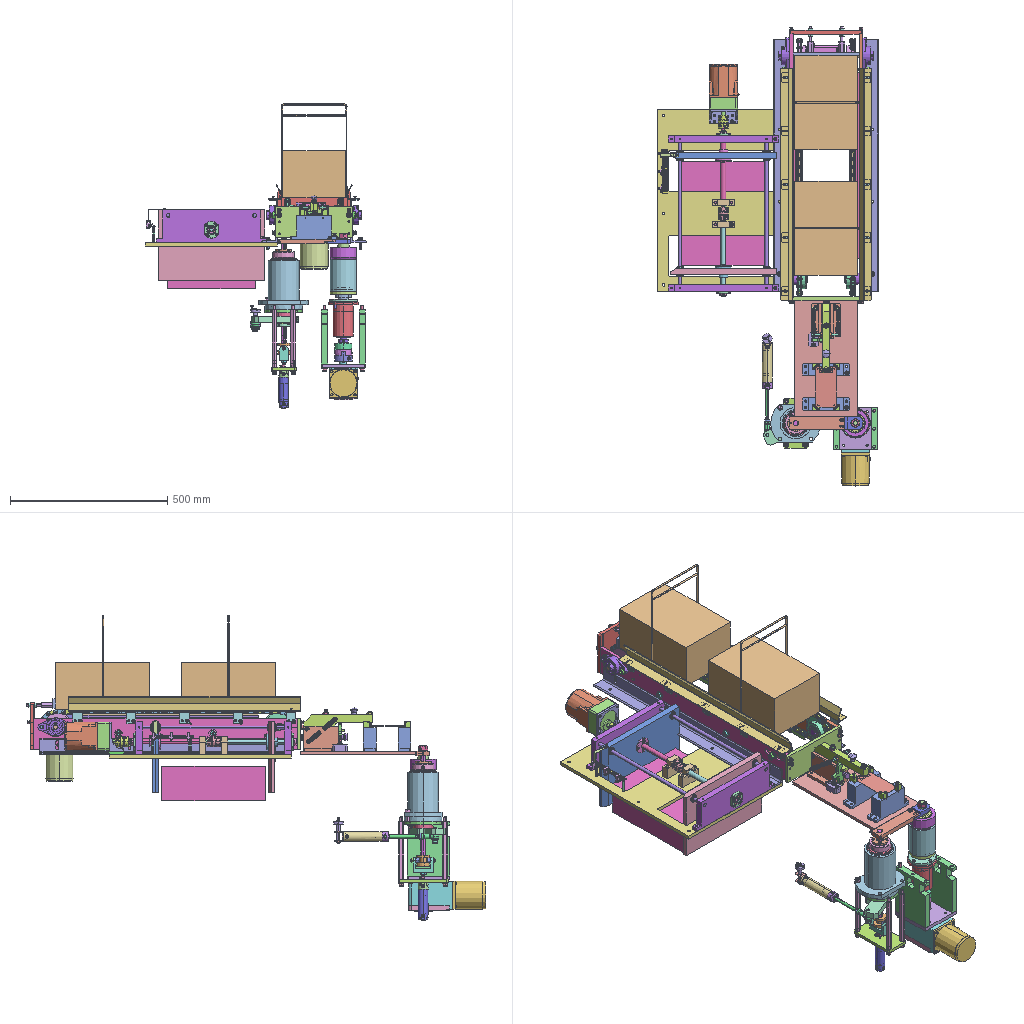Assembly | STEP file | 219 different items | 577 placed | box 704 x 1463 x 971 mm
Parts list (item | name | quantity | parent item | size | volume):
1 | 0217_205_Base_Plate | x1 | - | 200 x 370 x 10 mm | 736866 mm3
2 | 0217_207_Base | x2 | - | 150 x 40 x 75 mm | 343539 mm3
3 | 0217_017_WGDLJ-20-5-5 | x4 | - | 20 x 20 x 20 mm | 5354 mm3
4 | 0217_012_WSRPM20_40_20 | x1 | - | 40 x 20 x 5 mm | 3328 mm3
5 | 0217_002_WR18-20 | x2 | - | 19 x 4.5 x 19 mm | 92.511 mm3
6 | 0217_Z_AWA12-100 | x4 | in 0217_001_AWA12-100 | 13.1 x 13.1 x 53.1 mm | 757.901 mm3
7 | 0217_206_Base | x1 | in _0217_SA01 | 30 x 45 x 20 mm | 23102 mm3
8 | 0217_204_Block | x1 | in _0217_SA01 | 45 x 9.9 x 82 mm | 15419 mm3
9 | 0217_Z_PJL8-10-1 | x1 | in 0217_013_PJL8-10 | 43 x 8 x 8 mm | 1284 mm3
10 | 0217_Z_PJL8-10-2 | x1 | in 0217_013_PJL8-10 | 20 x 4.8 x 4.8 mm | 157.602 mm3
11 | 0217_003_DBTS6-10-10 | x1 | in _0217_SA01 | 24 x 16 x 16 mm | 1816 mm3
12 | 0217_301_SCB6-20 | x4 | in _0217_SA01, _0217_SA02 | 26 x 10 x 10 mm | 952.027 mm3
13 | 0217_306_SNTRCS8 | x1 | in _0217_SA01 | 4 x 15.011 x 13 mm | 435.9 mm3
14 | 0217_201_Base | x1 | in _0217_SA02 | 90 x 110 x 80 mm | 389355 mm3
15 | 0217_004_MPBZ15-10 | x2 | in _0217_SA02 | 10 x 21 x 21 mm | 1565 mm3
16 | 0217_Z_SBSP8-30-1 | x2 | in 0217_015_SBSPO8-30 | 30 x 8 x 8 mm | 1385 mm3
17 | 0217_Z_SBSP8-30-2 | x2 | in 0217_015_SBSPO8-30 | 6.8 x 15.011 x 13 mm | 746.792 mm3
18 | 0217_302_SLW6 | x3 | in _0217_SA02 | 1.5 x 12.2 x 12.2 mm | 128.756 mm3
19 | 0217_303_PFW6 | x3 | in _0217_SA02 | 1.6 x 12.5 x 12.5 mm | 141.61 mm3
20 | 0217_203_Shaft | x1 | in _0217_SA03 | 20 x 147 x 20 mm | 23227 mm3
21 | 0217_005_WSSS25-15-1 | x1 | in _0217_SA03 | 1 x 25 x 25 mm | 282.743 mm3
22 | 0217_006_WSSS25-8-1 | x1 | in _0217_SA03 | 1 x 25 x 25 mm | 414.69 mm3
23 | 0217_007_NOOS8-16 | x1 | in _0217_SA03 | 22 x 30 x 30 mm | 5015 mm3
24 | 0217_202_Arm | x1 | in _0217_SA04 | 20 x 220 x 54 mm | 161429 mm3
25 | 0217_016_MPFZU8-10 | x2 | in _0217_SA04 | 10 x 14 x 14 mm | 412.979 mm3
26 | 0217_Z_SBSPO8-45-1 | x2 | in 0217_014_SBSPO8-45 | 45 x 8 x 8 mm | 2139 mm3
27 | 0217_Z_SBSPO8-45-2 | x2 | in 0217_014_SBSPO8-45 | 6.8 x 15.011 x 13 mm | 746.792 mm3
28 | 0217_011_NMM6-25 | x1 | in _0217_SA04 | 25 x 32 x 25 mm | 5504 mm3
29 | 0217_Z_ANBNS10-80-1 | x1 | in 0217_010_ANBNS10_80 | 80 x 10 x 10 mm | 6095 mm3
30 | 0217_Z_ANBNS10-80-2 | x1 | in 0217_010_ANBNS10_80 | 6 x 19.6 x 17 mm | 1146 mm3
31 | 0217_Z_PUSS10-40-1 | x1 | in 0217_009_PUSS10-40 | 46 x 10 x 10 mm | 3323 mm3
32 | 0217_Z_PUSS10-40-2 | x1 | in 0217_009_PUSS10-40 | 6 x 19.63 x 17 mm | 1142 mm3
33 | 0217_Z_SCCG8-55-1 | x1 | in 0217_008_SCCG8-55 | 61 x 8 x 8 mm | 3039 mm3
34 | 0217_Z_SCCG8-55-2 | x2 | in 0217_008_SCCG8-55 | 0.8 x 14 x 11.95 mm | 51.564 mm3
35 | 0217_Work-A | x1 | - | 65 x 130 x 0.7 mm | 5915 mm3
36 | 0217_304_SCB3-25 | x4 | - | 28 x 5.5 x 5.5 mm | 238.258 mm3
37 | 0217_305_SFBJ6-12 | x1 | - | 12 x 12 x 12 mm | 419.433 mm3
38 | 0228_001_SRBN25-A | x4 | in _0228_SA01-1, _0228_SA01-2 | 25 x 1.6 x 25 mm | 333.381 mm3
39 | 0228_002_MSB12-25 | x4 | in _0228_SA01-1, _0228_SA01-2 | 45 x 17 x 17 mm | 5025 mm3
40 | 0228_Z_LGTS40-590-K4-P1601 | x2 | in 0228_006_LGTS40-590-K4-P160 | 17 x 14 x 590 mm | 119990 mm3
41 | 0228_Z_LGTS40-590-K4-P1602 | x2 | in 0228_006_LGTS40-590-K4-P160 | 20 x 10 x 590 mm | 38370 mm3
42 | 0228_007_STWN25 | x2 | in _0228_SA01-1, _0228_SA01-2 | 1.2 x 31.3 x 28.55 mm | 254.107 mm3
43 | 0228_009_SB6905ZZ | x4 | in _0228_SA01-1, _0228_SA01-2 | 9 x 42 x 42 mm | 7312 mm3
44 | 0228_Z_Chain_RF2040SSS-441 | x68 | in 0228_103_Chain_RF2040SSS-44 | 18.2 x 12 x 37.4 mm | 1630 mm3
45 | 0228_Z_Chain_RF2040SSS-442 | x68 | in 0228_103_Chain_RF2040SSS-44 | 10.95 x 12 x 37.4 mm | 1766 mm3
46 | 0228_104_Sprocket_RF2040S1200 | x2 | in _0228_SA01-1, _0228_SA01-2 | 103.209 x 103.209 x 25 mm | 105106 mm3
47 | 0228_105_Sprocket_RF2040S1200 | x2 | in _0228_SA01-1, _0228_SA01-2 | 103.209 x 103.209 x 25 mm | 79551 mm3
48 | 0228_201_Plate | x1 | in _0228_SA01-1 | 12 x 100 x 840 mm | 978760 mm3
49 | 0228_203_Bracket | x2 | in _0228_SA01-1, _0228_SA01-2 | 50 x 50 x 800 mm | 373941 mm3
50 | 0228_206_Guide | x2 | in _0228_SA01-1, _0228_SA01-2 | 6 x 18 x 600 mm | 64069 mm3
51 | 0228_207_Bracket | x2 | in _0228_SA01-1, _0228_SA01-2 | 30 x 30 x 590 mm | 100045 mm3
52 | 0228_210_Bracket | x10 | in _0228_SA01-1, _0228_SA01-2 | 25 x 40 x 30 mm | 5273 mm3
53 | 0228_211_Guide | x2 | in _0228_SA01-1, _0228_SA01-2 | 38 x 46.651 x 740 mm | 124477 mm3
54 | 0228_214_Shaft | x2 | in _0228_SA01-1, _0228_SA01-2 | 77.35 x 35 x 35 mm | 35572 mm3
55 | 0228_215_Post | x8 | in _0228_SA01-1, _0228_SA01-2 | 26 x 13.856 x 12 mm | 2134 mm3
56 | 0228_301_ACB8-100 | x2 | in _0228_SA01-1, _0228_SA01-2 | 108 x 13 x 13 mm | 5949 mm3
57 | socket head cap screw_iso_ISO 4762 M8 x 30 --- 30N | x2 | in _0228_SA01-1, _0228_SA01-2 | 38 x 13 x 13 mm | 2418 mm3
58 | socket head cap screw_iso_ISO 4762 M8 x 20 --- 20N | x2 | in _0228_SA01-1, _0228_SA01-2 | 28 x 13 x 13 mm | 1915 mm3
59 | 0228_305_MSSFS5-8 | x4 | in _0228_SA01-1, _0228_SA01-2 | 8 x 5 x 5 mm | 139.331 mm3
60 | 0228_308_SCB5-15 | x14 | in _0228_SA01-1, _0228_SA01-2 | 20 x 8.5 x 8.5 mm | 536.391 mm3
61 | socket head cap screw_iso_ISO 4762 M5 x 12 --- 12N | x2 | in _0228_SA01-1, _0228_SA01-2 | 17 x 8.5 x 8.5 mm | 476.406 mm3
62 | socket head cap screw_iso_ISO 4762 M4 x 8 --- 8N | x2 | in _0228_SA01-1, _0228_SA01-2 | 12 x 7 x 7 mm | 234.975 mm3
63 | 0228_311_LBNR12 | x2 | in _0228_SA01-1, _0228_SA01-2 | 10 x 21.9 x 19 mm | 2286 mm3
64 | 0228_313_SPWF12 | x2 | in _0228_SA01-1, _0228_SA01-2 | 2.5 x 24 x 24 mm | 799.143 mm3
65 | 0228_314_SPWF8 | x6 | in _0228_SA01-1, _0228_SA01-2 | 1.6 x 17 x 17 mm | 274.5 mm3
66 | 0228_316_SPWF5 | x14 | in _0228_SA01-1, _0228_SA01-2 | 1 x 10 x 10 mm | 56.478 mm3
67 | 0228_317_SPWF4 | x2 | in _0228_SA01-1, _0228_SA01-2 | 0.8 x 9 x 9 mm | 39.276 mm3
68 | 0228_318_SSLW12 | x2 | in _0228_SA01-1, _0228_SA01-2 | 3 x 21.5 x 21.494 mm | 721.153 mm3
69 | 0228_319_SSLW8 | x4 | in _0228_SA01-1, _0228_SA01-2 | 2 x 15.4 x 15.396 mm | 260.908 mm3
70 | 0228_321_SSLW5 | x16 | in _0228_SA01-1, _0228_SA01-2 | 1.3 x 9.2 x 9.198 mm | 58.481 mm3
71 | 0228_322_SSLW4 | x2 | in _0228_SA01-1, _0228_SA01-2 | 1 x 7.6 x 7.598 mm | 31.433 mm3
72 | 0228_202_Plate | x1 | in _0228_SA01-2 | 12 x 100 x 840 mm | 978079 mm3
73 | 0228_003_MSB12-10 | x1 | in _0228_SA02 | 30 x 17 x 17 mm | 3328 mm3
74 | 0228_004_SLSBG19-48-M10-N8 | x1 | in _0228_SA02 | 63 x 21.939 x 19 mm | 15277 mm3
75 | 0228_Z_HDH151 | x2 | in 0228_008_HDH15 | 113 x 60 x 33.3 mm | 71474 mm3
76 | 0228_Z_HDH152 | x2 | in 0228_008_HDH15 | 7.128 x 7.128 x 6 mm | 118.77 mm3
77 | 0228_Z_HDH153 | x2 | in 0228_008_HDH15 | 6 x 5 x 6 mm | 118.77 mm3
78 | 0228_010_KES5-25 | x3 | in _0228_SA02 | 25 x 5 x 5 mm | 594.343 mm3
79 | 0228_101_Motor_5RK40GN-C | x1 | in _0228_SA02 | 137 x 90 x 90 mm | 667092 mm3
80 | 0228_Z_Gearhead_5GN120RH1 | x1 | in 0228_102_Gearhead_5GN120RH | 107 x 104 x 93 mm | 637231 mm3
81 | 0228_Z_Gearhead_5GN120RH2 | x1 | in 0228_102_Gearhead_5GN120RH | 25 x 25 x 83 mm | 25062 mm3
82 | 0228_205_Shaft | x1 | in _0228_SA02 | 305 x 15 x 15 mm | 52825 mm3
83 | 0228_213_Arm | x1 | in _0228_SA02 | 9 x 78 x 135 mm | 88772 mm3
84 | socket head cap screw_iso_ISO 4762 M10 x 25 --- 25N | x2 | in _0228_SA02 | 35 x 16 x 16 mm | 3616 mm3
85 | socket head cap screw_iso_ISO 4762 M6 x 20 --- 20N | x5 | in _0228_SA02, _0228_Assy | 26 x 10 x 10 mm | 956.582 mm3
86 | 0228_315_SPWF6 | x5 | in _0228_SA02, _0228_Assy | 1.6 x 12.5 x 12.5 mm | 144.878 mm3
87 | 0228_320_SSLW6 | x5 | in _0228_SA02, _0228_Assy | 1.5 x 12.2 x 12.197 mm | 128.674 mm3
88 | 0228_005_SLSBH17-35-F50-M8-N6 | x2 | in _0228_Assy | 85 x 19.63 x 17 mm | 10911 mm3
89 | 0228_204_Shaft | x2 | in _0228_Assy | 210 x 20 x 20 mm | 61901 mm3
90 | 0228_208_Plate | x1 | in _0228_Assy | 234 x 150 x 12 mm | 410826 mm3
91 | 0228_209_Stopper | x1 | in _0228_Assy | 210 x 30 x 9 mm | 55294 mm3
92 | 0228_212_Plate | x1 | in _0228_Assy | 243 x 100 x 12 mm | 281737 mm3
93 | 0228_307_SCB6-15 | x2 | in _0228_Assy | 21 x 10 x 10 mm | 817.284 mm3
94 | 0228_312_SHNJ-M8 | x4 | in _0228_Assy | 6.5 x 15.011 x 13 mm | 713.151 mm3
95 | 0228_Work-A | x2 | in _0228_Assy | 209.998 x 299.999 x 300 mm | 9019523 mm3
96 | 0229_Z_SCSBS20-24_1 | x1 | in 0229_004_SCSBS20-24 | 32 x 32 x 15 mm | 5310 mm3
97 | 0229_Z_SCSBS20-24_2 | x1 | in 0229_004_SCSBS20-24 | 6 x 5 x 6 mm | 115.41 mm3
98 | 0229_Z_SCSBS20-24_3 | x1 | in 0229_004_SCSBS20-24 | 5 x 6 x 6 mm | 115.41 mm3
99 | 0229_Z_B6204ZZNR_1 | x2 | in 0229_007_B6204ZZNR | 14 x 47 x 47 mm | 18805 mm3
100 | 0229_Z_B6204ZZNR_2 | x2 | in 0229_007_B6204ZZNR | 1.12 x 52.6 x 52.7 mm | 674.018 mm3
101 | 0229_Z_MFJC55-20-22_1 | x1 | in 0229_010_MFJC55-20-22 | 17 x 55 x 55 mm | 22049 mm3
102 | 0229_Z_MFJC55-20-22_2 | x1 | in 0229_010_MFJC55-20-22 | 30 x 55 x 54.982 mm | 40722 mm3
103 | 0229_Z_MFJC55-20-22_3 | x1 | in 0229_010_MFJC55-20-22 | 10 x 30.82 x 10 mm | 1082 mm3
104 | 0229_Z_MFJC55-20-22_4 | x1 | in 0229_010_MFJC55-20-22 | 30 x 54.982 x 55 mm | 39507 mm3
105 | 0229_Z_MFJC55-20-22_5 | x1 | in 0229_010_MFJC55-20-22 | 10 x 10 x 30.82 mm | 1082 mm3
106 | 0229_Z_5IK40AW-GAL20J_1 | x1 | in 0229_101_Servo_Motor_5IK40AW-GAL20J | 150 x 90 x 140 mm | 1226880 mm3
107 | 0229_Z_5IK40AW-GAL20J_2 | x1 | in 0229_101_Servo_Motor_5IK40AW-GAL20J | 90 x 93.5 x 105 mm | 664924 mm3
108 | 0229_201_Plate | x1 | in _0229_SA01 | 135 x 12 x 140 mm | 188675 mm3
109 | 0229_202_Plate | x2 | in _0229_SA01 | 135 x 173 x 20 mm | 406809 mm3
110 | 0229_211_Holder | x1 | in _0229_SA01 | 95 x 110 x 95 mm | 199422 mm3
111 | 0229_213_Shaft | x1 | in _0229_SA01 | 50 x 184 x 50 mm | 77662 mm3
112 | 0229_214_Holder | x1 | in _0229_SA01 | 85 x 10 x 85 mm | 51385 mm3
113 | 0229_215_Holder | x1 | in _0229_SA01 | 78 x 22 x 78 mm | 64740 mm3
114 | 0229_220_Holder | x1 | in _0229_SA01 | 89 x 8 x 89 mm | 33937 mm3
115 | 0229_302_M5x12 | x1 | in _0229_SA01 | 17 x 8.5 x 8.5 mm | 476.423 mm3
116 | 0229_306_M6x16 | x1 | in _0229_SA01 | 22 x 10 x 10 mm | 843.509 mm3
117 | 0229_307_M6x20 | x2 | in _0229_SA01 | 26 x 10 x 10 mm | 956.605 mm3
118 | 0229_309_M8x30 | x4 | in _0229_SA01 | 38 x 13 x 13 mm | 2418 mm3
119 | 0229_315_SPWF8 | x8 | in _0229_SA01, _0229_SA02 | 1.6 x 17 x 17 mm | 274.5 mm3
120 | 0229_317_SSLW6 | x2 | in _0229_SA01, _0229_SA02 | 1.5 x 12.2 x 12.197 mm | 128.674 mm3
121 | 0229_318_SSLW8 | x8 | in _0229_SA01, _0229_SA02 | 2 x 15.4 x 15.396 mm | 260.908 mm3
122 | 0229_Z_PHSC10A_1 | x1 | in 0229_001_PHSC10A | - | 7061 mm3
123 | 0229_Z_PHSC10A_2 | x1 | in 0229_001_PHSC10A | - | 2169 mm3
124 | 0229_Z_CFUA6-16_1 | x2 | in 0229_002_CFUA6-16 | 28 x 15.999 x 16 mm | 2735 mm3
125 | 0229_Z_CFUA6-16_2 | x2 | in 0229_002_CFUA6-16 | 5.2 x 11.547 x 10 mm | 345.697 mm3
126 | 0229_Z_SCCN50-22_1 | x1 | in 0229_003_SCCN50-22 | 22 x 70 x 70 mm | 36768 mm3
127 | 0229_Z_SCCN50-22_2 | x1 | in 0229_003_SCCN50-22 | 10 x 8 x 10 mm | 459 mm3
128 | 0229_Z_SCCN50-22_3 | x1 | in 0229_003_SCCN50-22 | 10 x 10 x 8 mm | 459.001 mm3
129 | 0229_005_STWN30 | x1 | in _0229_SA02 | 1.5 x 36.9 x 33.85 mm | 424.063 mm3
130 | 0229_006_STWN10 | x1 | in _0229_SA02 | 1 x 14.4 x 12.3 mm | 59.275 mm3
131 | 0229_Z_B6010ZZNR_1 | x2 | in 0229_008_B6010ZZNR | 16 x 80 x 80 mm | 45982 mm3
132 | 0229_Z_B6010ZZNR_2 | x2 | in 0229_008_B6010ZZNR | 1.7 x 86.435 x 86.6 mm | 2077 mm3
133 | 0229_009_B6206ZZ | x2 | in _0229_SA02 | 16 x 62 x 62 mm | 35690 mm3
134 | 0229_Z_BSFM16-335-M8-NTW_1 | x1 | in 0229_011_BSFM16-335-M8-NTW | 16.6 x 16.559 x 335 mm | 69757 mm3
135 | 0229_Z_BSFM16-335-M8-NTW_2 | x1 | in 0229_011_BSFM16-335-M8-NTW | 51 x 51 x 50 mm | 33822 mm3
136 | 0229_Z_BSFM16-335-M8-NTW_3 | x1 | in 0229_011_BSFM16-335-M8-NTW | 51 x 51 x 50 mm | 33822 mm3
137 | 0229_Z_Cylinder_CG1BN25-50_1 | x1 | in 0229_102_Cylinder_CG1BN25-50 | 31 x 100 x 31 mm | 43980 mm3
138 | 0229_Z_Cylinder_CG1BN25-50_2 | x1 | in 0229_102_Cylinder_CG1BN25-50 | 31.4 x 23 x 31.4 mm | 12893 mm3
139 | 0229_Z_Cylinder_CG1BN25-50_3 | x1 | in 0229_102_Cylinder_CG1BN25-50 | 24.9 x 137.5 x 24.9 mm | 12725 mm3
140 | 0229_Z_Cylinder_CG1BN25-50_4 | x1 | in 0229_102_Cylinder_CG1BN25-50 | 19.6 x 6 x 17 mm | 1151 mm3
141 | 0229_Z_Cylinder_CG1DN25-75_1 | x1 | in 0229_103_Cylinder_CG1DN25-75 | 31 x 31 x 125 mm | 50538 mm3
142 | 0229_Z_Cylinder_CG1DN25-75_2 | x1 | in 0229_103_Cylinder_CG1DN25-75 | 31.4 x 31.4 x 23 mm | 12832 mm3
143 | 0229_Z_Cylinder_CG1DN25-75_3 | x1 | in 0229_103_Cylinder_CG1DN25-75 | 24.9 x 24.9 x 162.5 mm | 14688 mm3
144 | 0229_Z_Cylinder_CG1DN25-75_4 | x1 | in 0229_103_Cylinder_CG1DN25-75 | 33 x 31 x 29 mm | 5061 mm3
145 | 0229_Z_Cylinder_CG1DN25-75_5 | x1 | in 0229_103_Cylinder_CG1DN25-75 | 19.6 x 6 x 17 mm | 1151 mm3
146 | 0229_203_Plate | x1 | in _0229_SA02 | 160 x 10 x 80 mm | 122466 mm3
147 | 0229_204_Stud | x4 | in _0229_SA02 | 16.166 x 198.5 x 14 mm | 31042 mm3
148 | 0229_205_Joint | x1 | in _0229_SA02 | 64 x 48 x 30 mm | 41736 mm3
149 | 0229_206_Joint | x1 | in _0229_SA02 | 40 x 35 x 40 mm | 25414 mm3
150 | 0229_207_Pin | x1 | in _0229_SA02 | 30 x 73 x 30 mm | 11176 mm3
151 | 0229_208_Holder | x1 | in _0229_SA02 | 120 x 10 x 120 mm | 60495 mm3
152 | 0229_209_Color | x1 | in _0229_SA02 | 56 x 15.2 x 56 mm | 7593 mm3
153 | 0229_210_Holder | x1 | in _0229_SA02 | 120 x 157 x 160 mm | 628932 mm3
154 | 0229_212_Holder | x1 | in _0229_SA02 | 50 x 230 x 50 mm | 276670 mm3
155 | 0229_216_Holder | x1 | in _0229_SA02 | 85 x 45 x 85 mm | 112200 mm3
156 | 0229_217_Arm | x1 | in _0229_SA02 | 70 x 20 x 150 mm | 127979 mm3
157 | 0229_218_Arm | x1 | in _0229_SA02 | 40 x 15 x 176.5 mm | 91943 mm3
158 | 0229_219_Arm | x1 | in _0229_SA02 | 40 x 15 x 77 mm | 33260 mm3
159 | 0229_221_Pin | x1 | in _0229_SA02 | 36 x 89 x 36 mm | 38557 mm3
160 | 0229_301_M4x10 | x2 | in _0229_SA02 | 14 x 7 x 7 mm | 260.117 mm3
161 | 0229_303_SCB5-15 | x1 | in _0229_SA02 | 20 x 8.5 x 8.5 mm | 536.391 mm3
162 | 0229_304_M5x16 | x1 | in _0229_SA02 | 21 x 8.5 x 8.5 mm | 554.961 mm3
163 | 0229_305_SCB6-15 | x2 | in _0229_SA02 | 21 x 10 x 10 mm | 817.284 mm3
164 | 0229_308_M6x40 | x1 | in _0229_SA02 | 46 x 10 x 10 mm | 1522 mm3
165 | 0229_310_M8x25 | x4 | in _0229_SA02 | 33 x 13 x 13 mm | 2167 mm3
166 | 0229_311_M8x35 | x1 | in _0229_SA02 | 43 x 13 x 13 mm | 2669 mm3
167 | 0229_312_M8x45 | x1 | in _0229_SA02 | 53 x 13 x 13 mm | 3172 mm3
168 | 0229_313_M10x30 | x1 | in _0229_SA02 | 40 x 16 x 16 mm | 4009 mm3
169 | 0229_314_M10x40 | x1 | in _0229_SA02 | 50 x 16 x 16 mm | 4794 mm3
170 | 0229_316_SPWF10 | x1 | in _0229_SA02 | 2 x 21 x 21 mm | 519.541 mm3
171 | 0229_319_SSLW10 | x1 | in _0229_SA02 | 2.5 x 18.4 x 18.395 mm | 449.851 mm3
172 | 0229_320_SSLW16 | x1 | in _0229_SA02 | 4 x 28 x 27.992 mm | 1600 mm3
173 | 0229_321_SLBNR16 | x1 | in _0229_SA02 | 13 x 27.7 x 24 mm | 4462 mm3
174 | 0229_Work-A | x1 | in _0229_Assy | 85 x 102 x 85 mm | 125379 mm3
175 | 0230_201_Base | x1 | in _0230_Assy | 420 x 12 x 579.7 mm | 1822838 mm3
176 | 0230_204_Block | x2 | in _0230_Assy | 350 x 104 x 20 mm | 627795 mm3
177 | 0230_Z_005_MRWZ12_1 | x2 | in 0230_005_MRWZ12 | 44 x 54 x 24 mm | 16765 mm3
178 | 0230_Z_005_MRWZ12_2 | x2 | in 0230_005_MRWZ12 | 30 x 30 x 4.8 mm | 1915 mm3
179 | 0230_Z_005_MRWZ12_3 | x2 | in 0230_005_MRWZ12 | 15 x 15 x 5 mm | 318.086 mm3
180 | 0230_Z_005_MRWZ12_4 | x4 | in 0230_005_MRWZ12 | 28 x 28 x 8 mm | 3776 mm3
181 | 0230_Z_005_MRWZ12_5 | x2 | in 0230_005_MRWZ12 | 22 x 22 x 8 mm | 1767 mm3
182 | 0230_Z_005_MRWZ12_6 | x2 | in 0230_005_MRWZ12 | 4 x 4 x 4 mm | 41.33 mm3
183 | 0230_006_MTUZ12 | x2 | in _0230_Assy | 70 x 58 x 20 mm | 55020 mm3
184 | 0230_011_SSFJ12-495 | x2 | in _0230_Assy | 12 x 12 x 495 mm | 55974 mm3
185 | 0230_205_Plate | x1 | in _0230_SA01 | 90 x 8 x 46 mm | 32215 mm3
186 | 0230_Z_007_CPLCN32-12-12_1 | x1 | in 0230_007_CPLCN32-12-12 | 41 x 32 x 32 mm | 22249 mm3
187 | 0230_Z_007_CPLCN32-12-12_1_2 | x4 | in 0230_007_CPLCN32-12-12 | 7 x 7 x 13.82 mm | 252.508 mm3
188 | 0230_Z_008_CPLCN32-10-12_1 | x1 | in 0230_008_CPLCN32-10-12 | 41 x 32 x 32 mm | 22644 mm3
189 | 0230_Z_008_CPLCN32-10-12_2 | x4 | in 0230_008_CPLCN32-10-12 | 7 x 7 x 13.82 mm | 252.508 mm3
190 | 0230_009_KNCLB12-16-10 | x2 | in _0230_SA01 | 10 x 16 x 16 mm | 876.127 mm3
191 | 0230_Z_013_PACMR90-W40-V100-MTB90_1 | x1 | in 0230_013_PACMR90-W40-V100-MTB90 | 105 x 90 x 95 mm | 733234 mm3
192 | 0230_Z_013_PACMR90-W40-V100-MTB90_2 | x1 | in 0230_013_PACMR90-W40-V100-MTB90 | 46 x 95 x 90 mm | 55942 mm3
193 | 0230_Z_014_PACMGX90-3_1 | x1 | in 0230_014_PACMGX90-3 | 69 x 90 x 90 mm | 301887 mm3
194 | 0230_001_MTSRK16-275-F30-R12-T30-Q12-S20-E10-BQ15 | x1 | in _0230_SA01 | 16 x 16 x 275 mm | 47560 mm3
195 | 0230_002_MTSLW16-255-F30-V12-S30-Q12-BV15 | x1 | in _0230_SA01 | 16 x 16 x 255 mm | 45988 mm3
196 | 0230_305_SCB6-55 | x1 | in _0230_SA01 | 61 x 10 x 10 mm | 1947 mm3
197 | 0230_306_SCB6-25 | x1 | in _0230_SA01 | 31 x 10 x 10 mm | 1100 mm3
198 | 0230_307_SLW6 | x1 | in _0230_SA01 | 1.5 x 12.2 x 12.197 mm | 128.674 mm3
199 | 0230_308_PFW6 | x1 | in _0230_SA01 | 1.6 x 12.5 x 12.5 mm | 144.878 mm3
200 | 0230_202_Guide | x1 | in _0230_SA02 | 340 x 226 x 20.4 mm | 1516540 mm3
201 | 0230_206_Bracket | x1 | in _0230_SA02 | 57 x 39.5 x 10 mm | 940.863 mm3
202 | 0230_003_MTSFR16 | x1 | in _0230_SA02 | 35 x 51 x 51 mm | 24500 mm3
203 | 0230_010_LMUF12 | x4 | in _0230_SA02, _0230_SA03 | 30 x 21 x 21 mm | 6897 mm3
204 | 0230_012_STWN21 | x8 | in _0230_SA02, _0230_SA03 | 1.2 x 26.7 x 24.05 mm | 188.679 mm3
205 | 0230_309_SCB3-6 | x2 | in _0230_SA02, _0230_SA04 | 9 x 5.5 x 5.5 mm | 103.858 mm3
206 | 0230_310_SCB6-16 | x2 | in _0230_SA02, _0230_SA03 | 22 x 10 x 10 mm | 845.558 mm3
207 | 0230_203_Guide | x1 | in _0230_SA03 | 340 x 226 x 20.4 mm | 1516641 mm3
208 | 0230_004_MTSFL16 | x1 | in _0230_SA03 | 35 x 51 x 51 mm | 24500 mm3
209 | 0230_016_SENBF3-140 | x1 | in _0230_SA04 | 140 x 16 x 9 mm | 7179 mm3
210 | 0230_015_FPMT54 | x3 | in _0230_SA04 | 13.7 x 27.2 x 26 mm | 2173 mm3
211 | 0230_017_LSBWRK6-50 | x2 | in _0230_SA04 | 6.928 x 54.5 x 6 mm | 1554 mm3
212 | 0230_311_SCB3-8 | x3 | in _0230_SA04 | 11 x 5.5 x 5.5 mm | 117.995 mm3
213 | 0230_312_SLW3 | x3 | in _0230_SA04 | 0.7 x 5.9 x 5.898 mm | 13.546 mm3
214 | 0230_313_PFW3 | x3 | in _0230_SA04 | 0.8 x 6 x 6 mm | 16.185 mm3
215 | 0230_Work-A | x1 | in _0230_Assy | 280 x 110 x 330 mm | 10164000 mm3
216 | 0230_301_MMSU5-10 | x2 | in _0230_Assy | 10 x 5 x 5 mm | 171.124 mm3
217 | 0230_302_SCB4-10 | x2 | in _0230_Assy | 14 x 7 x 7 mm | 260.298 mm3
218 | 0230_303_SCB6-20 | x2 | in _0230_Assy | 26 x 10 x 10 mm | 958.655 mm3
219 | 0230_304_SCB8-45 | x1 | in _0230_Assy | 53 x 13 x 13 mm | 3170 mm3
Placements (level | parent | child | x y z in mm | rotation matrix by rows), first 233 of 630 lines:
1 | subassembly 2 | 0217_205_Base_Plate | -95.531 -185.789 -5.0 | 1 0 0 0 1 0 0 0 1
1 | subassembly 2 | 0217_207_Base | 4.469 -165.789 5.0 | 1 0 0 0 1 0 0 0 1
1 | subassembly 2 | 0217_207_Base | 4.469 -15.789 5.0 | -1 0 0 0 -1 0 0 0 1
1 | subassembly 2 | 0217_017_WGDLJ-20-5-5 | 46.969 -15.789 80.0 | 0 0 -1 -1 0 0 0 1 0
1 | subassembly 2 | 0217_017_WGDLJ-20-5-5 | -38.031 -15.789 80.0 | 1 0 0 0 0 -1 0 1 0
1 | subassembly 2 | 0217_017_WGDLJ-20-5-5 | 46.969 -165.789 80.0 | -1 0 0 0 0 1 0 1 0
1 | subassembly 2 | 0217_017_WGDLJ-20-5-5 | -38.031 -165.789 80.0 | 0 0 1 1 0 0 0 1 0
1 | subassembly 2 | 0217_012_WSRPM20_40_20 | -15.531 -45.789 80.0 | 1 0 0 0 1 0 0 0 1
1 | subassembly 2 | 0217_002_WR18-20 | 4.469 179.211 50.0 | 0.8372 0 -0.5469 0 1 0 0.5469 0 0.8372
1 | subassembly 2 | 0217_002_WR18-20 | 4.469 179.211 50.0 | -0.8372 0 -0.5469 0 -1 0 -0.5469 0 0.8372
1 | subassembly 2 | 0217_001_AWA12-100 | -34.125 91.463 91.856 | 1 0 0 0 0.6463 -0.763 0 0.763 0.6463
2 | 0217_001_AWA12-100 | 0217_Z_AWA12-100 | -1.906 0.4047 14.002 | 1 0 0 0 1 0 0 0 1
2 | 0217_001_AWA12-100 | 0217_Z_AWA12-100 | -1.906 0.4047 -79.494 | 1 0 0 0 -1 0 0 0 -1
1 | subassembly 2 | 0217_001_AWA12-100 | 45.469 91.518 91.919 | 1 0 0 0 0.6436 -0.7654 0 0.7654 0.6436
2 | 0217_001_AWA12-100 | 0217_Z_AWA12-100 | -1.906 0.4047 14.002 | 1 0 0 0 1 0 0 0 1
2 | 0217_001_AWA12-100 | 0217_Z_AWA12-100 | -1.906 0.4047 -79.493 | 1 0 0 0 -1 0 0 0 -1
1 | subassembly 2 | _0217_SA01 | -30.448 60.714 15.0 | 1 0 0 0 1 0 0 0 1
2 | _0217_SA01 | 0217_206_Base | -5.083 -24.003 -10.0 | 1 0 0 0 1 0 0 0 1
2 | _0217_SA01 | 0217_204_Block | 35.17 -6.503 -4.74 | 0.9997 0 -0.02564 0 1 0 0.02564 0 0.9997
2 | _0217_SA01 | 0217_013_PJL8-10 | 1.695 -0.287 18.417 | 0 0 1 0 1 0 -1 0 0
3 | 0217_013_PJL8-10 | 0217_Z_PJL8-10-1 | -12.583 -1.216 -6.778 | 1 0 0 0 1 0 0 0 1
3 | 0217_013_PJL8-10 | 0217_Z_PJL8-10-2 | -8.824 -1.216 -6.778 | 1 0 0 0 0.4105 0.9119 0 -0.9119 0.4105
2 | _0217_SA01 | 0217_003_DBTS6-10-10 | 24.917 -6.503 5.0 | 0 -1 0 1 0 0 0 0 1
2 | _0217_SA01 | 0217_301_SCB6-20 | -5.083 -16.503 3.4 | 0 0 1 0 1 0 -1 0 0
2 | _0217_SA01 | 0217_306_SNTRCS8 | -5.083 -1.503 14.0 | 0 0.14 0.9901 0 0.9901 -0.14 -1 0 0
1 | subassembly 2 | _0217_SA02 | 5.797 121.165 45.0 | 1 0 0 0 1 0 0 0 1
2 | _0217_SA02 | 0217_201_Base | -1.329 -56.954 -40.0 | 1 0 0 0 1 0 0 0 1
2 | _0217_SA02 | 0217_004_MPBZ15-10 | -1.329 53.046 5.0 | 0 0.133 -0.9911 -1 0 0 0 0.9911 0.133
2 | _0217_SA02 | 0217_004_MPBZ15-10 | -1.329 -41.954 5.0 | 0 -0.9974 0.07137 1 0 0 0 0.07137 0.9974
2 | _0217_SA02 | 0217_015_SBSPO8-30 | -46.764 38.545 -8.314 | 1 0 0 0 0.866 -0.5 0 0.5 0.866
3 | 0217_015_SBSPO8-30 | 0217_Z_SBSP8-30-1 | -0.0646 -1.275 -1.211 | 1 0 0 0 1 0 0 0 1
3 | 0217_015_SBSPO8-30 | 0217_Z_SBSP8-30-2 | -1.365 -1.275 -1.211 | 1 0 0 0 0.866 -0.5 0 0.5 0.866
2 | _0217_SA02 | 0217_015_SBSPO8-30 | 44.107 36.337 -9.589 | -1 0 0 0 -0.866 -0.5 0 -0.5 0.866
3 | 0217_015_SBSPO8-30 | 0217_Z_SBSP8-30-1 | -0.0646 -1.275 -1.211 | 1 0 0 0 1 0 0 0 1
3 | 0217_015_SBSPO8-30 | 0217_Z_SBSP8-30-2 | -1.365 -1.275 -1.211 | 1 0 0 0 0.866 -0.5 0 0.5 0.866
2 | _0217_SA02 | 0217_301_SCB6-20 | 33.672 -26.954 -26.9 | 0 0 1 0 1 0 -1 0 0
2 | _0217_SA02 | 0217_302_SLW6 | 33.672 -26.954 -26.9 | 0 0 1 0 1 0 -1 0 0
2 | _0217_SA02 | 0217_303_PFW6 | 33.672 -26.954 -28.4 | 0 0 1 0 1 0 -1 0 0
1 | subassembly 2 | _0217_SA03 | 9.795 119.67 50.0 | 1 0 0 0 1 0 0 0 1
2 | _0217_SA03 | 0217_203_Shaft | -5.326 -65.459 -0.0 | 1 0 0 0 1 0 0 0 1
2 | _0217_SA03 | 0217_005_WSSS25-15-1 | -5.326 55.541 0.0 | 0 0.1392 0.9903 -1 0 0 0 -0.9903 0.1392
2 | _0217_SA03 | 0217_006_WSSS25-8-1 | -5.326 64.541 -0.0 | 0 1 0 -1 0 0 0 0 1
2 | _0217_SA03 | 0217_007_NOOS8-16 | -5.326 64.541 -0.0 | 0 -0.8248 -0.5654 -1 0 0 0 0.5654 -0.8248
1 | subassembly 2 | _0217_SA04 | 15.878 62.492 94.0 | 1 0 0 0 1 0 0 0 1
2 | _0217_SA04 | 0217_202_Arm | -11.409 111.719 -27.0 | 1 0 0 0 1 0 0 0 1
2 | _0217_SA04 | 0217_016_MPFZU8-10 | -23.41 101.719 -19.0 | 1 0 0 0 1 0 0 0 1
2 | _0217_SA04 | 0217_016_MPFZU8-10 | 0.5905 101.719 -19.0 | -1 0 0 0 0.6732 -0.7394 0 -0.7394 -0.6732
2 | _0217_SA04 | 0217_014_SBSPO8-45 | -34.858 11.67 14.04 | 1 0 0 0 0.866 -0.5 0 0.5 0.866
3 | 0217_014_SBSPO8-45 | 0217_Z_SBSPO8-45-1 | -22.052 -0.4773 -0.9255 | 1 0 0 0 1 0 0 0 1
3 | 0217_014_SBSPO8-45 | 0217_Z_SBSPO8-45-2 | -23.352 -0.4773 -0.9255 | 1 0 0 0 0.866 -0.5 0 0.5 0.866
2 | _0217_SA04 | 0217_014_SBSPO8-45 | 12.039 12.595 12.437 | -1 0 0 0 0.866 0.5 0 0.5 -0.866
3 | 0217_014_SBSPO8-45 | 0217_Z_SBSPO8-45-1 | -22.052 -0.4773 -0.9255 | 1 0 0 0 1 0 0 0 1
3 | 0217_014_SBSPO8-45 | 0217_Z_SBSPO8-45-2 | -23.352 -0.4773 -0.9255 | 1 0 0 0 0.866 -0.5 0 0.5 0.866
2 | _0217_SA04 | 0217_011_NMM6-25 | -11.409 -48.281 27.0 | 1 0 0 0 0 -1 0 1 0
2 | _0217_SA04 | 0217_010_ANBNS10_80 | -9.92 38.808 38.78 | 0 0.1301 0.9915 0 0.9915 -0.1301 -1 0 0
3 | 0217_010_ANBNS10_80 | 0217_Z_ANBNS10-80-1 | -4.22 2.693 -1.855 | 1 0 0 0 1 0 0 0 1
3 | 0217_010_ANBNS10_80 | 0217_Z_ANBNS10-80-2 | 48.78 2.693 -1.855 | -1 0 0 0 0.3818 -0.9242 0 -0.9242 -0.3818
2 | _0217_SA04 | 0217_009_PUSS10-40 | -11.209 -99.868 -1.317 | 0 0.866 0.5 0 -0.5 0.866 1 0 0
3 | 0217_009_PUSS10-40 | 0217_Z_PUSS10-40-1 | -0.9827 -0.9669 1.275 | 1 0 0 0 1 0 0 0 1
3 | 0217_009_PUSS10-40 | 0217_Z_PUSS10-40-2 | 11.317 -0.9669 1.275 | 1 0 0 0 1 0 0 0 1
2 | _0217_SA04 | 0217_008_SCCG8-55 | -11.409 101.719 -19.0 | 1 0 0 0 0.7562 0.6543 0 -0.6543 0.7562
3 | 0217_008_SCCG8-55 | 0217_Z_SCCG8-55-1 | -30.5 -0.0 -0.0 | 1 0 0 0 1 0 0 0 1
3 | 0217_008_SCCG8-55 | 0217_Z_SCCG8-55-2 | -30.5 -0.0 -0.0 | 1 0 0 0 1 0 0 0 1
3 | 0217_008_SCCG8-55 | 0217_Z_SCCG8-55-2 | 25.4 -0.0 -0.0 | 1 0 0 0 1 0 0 0 1
1 | subassembly 2 | 0217_Work-A | 4.469 -155.789 85.0 | 1 0 0 0 1 0 0 0 1
1 | subassembly 2 | 0217_301_SCB6-20 | 69.469 -45.789 18.1 | 0 0 1 0 1 0 -1 0 0
1 | subassembly 2 | 0217_301_SCB6-20 | 69.469 -155.789 18.1 | 0 0 1 0 1 0 -1 0 0
1 | subassembly 2 | 0217_302_SLW6 | 69.469 -155.789 18.1 | 0 0 1 0 1 0 -1 0 0
1 | subassembly 2 | 0217_302_SLW6 | 69.469 -45.789 18.1 | 0 0 1 0 1 0 -1 0 0
1 | subassembly 2 | 0217_303_PFW6 | 69.469 -155.789 16.6 | 0 0 1 0 1 0 -1 0 0
1 | subassembly 2 | 0217_303_PFW6 | 69.469 -45.789 16.6 | 0 0 1 0 1 0 -1 0 0
1 | subassembly 2 | 0217_304_SCB3-25 | 43.469 -150.789 96.5 | 0 0 1 0 1 0 -1 0 0
1 | subassembly 2 | 0217_304_SCB3-25 | -34.531 -30.789 96.5 | 0 0 1 0 1 0 -1 0 -0
1 | subassembly 2 | 0217_304_SCB3-25 | -34.531 -150.789 96.5 | 0 0 1 0 1 0 -1 0 -0
1 | subassembly 2 | 0217_304_SCB3-25 | 43.469 -30.789 96.5 | 0 0 1 0 1 0 -1 0 -0
1 | subassembly 2 | 0217_305_SFBJ6-12 | 14.469 -35.789 81.6 | 1 0 0 0 1 0 0 0 1
1 | subassembly 2 | _0228_Assy | 115.469 194.211 10.0 | 1 0 0 0 0 -1 0 1 0
2 | _0228_Assy | _0228_SA01-1 | -0.0 -0.0 -0.0 | 1 0 0 0 1 0 0 0 1
3 | _0228_SA01-1 | 0228_001_SRBN25-A | 6.006 52.0 -270.0 | 0 1 0 1 0 0 0 0 -1
3 | _0228_SA01-1 | 0228_001_SRBN25-A | 6.006 52.0 -570.0 | 0 1 0 -0.8443 0 0.5359 0.5359 0 0.8443
3 | _0228_SA01-1 | 0228_002_MSB12-25 | 7.6 52.0 -270.0 | -1 0 0 0 0.5 -0.866 0 -0.866 -0.5
3 | _0228_SA01-1 | 0228_002_MSB12-25 | 7.6 52.0 -570.0 | -1 0 0 0 1 0 0 0 -1
3 | _0228_SA01-1 | 0228_006_LGTS40-590-K4-P160 | -26.0 103.0 -125.0 | 1 0 0 0 1 0 0 0 1
4 | 0228_006_LGTS40-590-K4-P160 | 0228_Z_LGTS40-590-K4-P1601 | -0.0 0.0 -0.0 | 1 0 0 0 1 0 0 0 1
4 | 0228_006_LGTS40-590-K4-P160 | 0228_Z_LGTS40-590-K4-P1602 | -0.0 -3.0 -0.0 | 1 0 0 0 1 0 0 0 1
3 | _0228_SA01-1 | 0228_007_STWN25 | -48.1 72.0 -58.81 | 1 0 0 0 1 0 0 0 1
3 | _0228_SA01-1 | 0228_009_SB6905ZZ | -47.35 72.0 -58.81 | 1 0 0 0 1 0 0 0 1
3 | _0228_SA01-1 | 0228_009_SB6905ZZ | -31.35 72.0 -58.81 | 1 0 0 0 1 0 0 0 1
3 | _0228_SA01-1 | 0228_103_Chain_RF2040SSS-44 | -26.0 72.0 -770.0 | -1 0 0 0 1 0 0 0 -1
4 | 0228_103_Chain_RF2040SSS-44 | 0228_Z_Chain_RF2040SSS-441 | 0.0 24.548 42.489 | 1 0 0 0 0.7073 -0.7069 0 0.7069 0.7073
4 | 0228_103_Chain_RF2040SSS-44 | 0228_Z_Chain_RF2040SSS-441 | -0.0 49.07 -50.8 | 1 0 0 0 1 0 0 0 1
4 | 0228_103_Chain_RF2040SSS-44 | 0228_Z_Chain_RF2040SSS-441 | 0.0 49.07 -101.6 | 1 0 0 0 1 0 0 0 1
4 | 0228_103_Chain_RF2040SSS-44 | 0228_Z_Chain_RF2040SSS-442 | 0.0 42.503 24.523 | 1 0 0 0 0.966 -0.2585 0 0.2585 0.966
4 | 0228_103_Chain_RF2040SSS-44 | 0228_Z_Chain_RF2040SSS-442 | 0.0 49.07 -76.2 | 1 0 0 0 1 0 0 0 1
4 | 0228_103_Chain_RF2040SSS-44 | 0228_Z_Chain_RF2040SSS-442 | 0.0 49.07 -127.0 | 1 0 0 0 1 0 0 0 1
4 | 0228_103_Chain_RF2040SSS-44 | 0228_Z_Chain_RF2040SSS-442 | -0.0 49.07 -177.8 | 1 0 0 0 1 0 0 0 1
4 | 0228_103_Chain_RF2040SSS-44 | 0228_Z_Chain_RF2040SSS-442 | 0.0 49.07 -228.6 | 1 0 0 0 1 0 0 0 1
4 | 0228_103_Chain_RF2040SSS-44 | 0228_Z_Chain_RF2040SSS-442 | -0.0 49.07 -279.4 | 1 0 0 0 1 0 0 0 1
4 | 0228_103_Chain_RF2040SSS-44 | 0228_Z_Chain_RF2040SSS-442 | 0.0 49.07 -330.2 | 1 0 0 0 1 0 0 0 1
4 | 0228_103_Chain_RF2040SSS-44 | 0228_Z_Chain_RF2040SSS-442 | 0.0 49.07 -381.0 | 1 0 0 0 1 0 0 0 1
4 | 0228_103_Chain_RF2040SSS-44 | 0228_Z_Chain_RF2040SSS-442 | 0.0 49.07 -431.8 | 1 0 0 0 1 0 0 0 1
4 | 0228_103_Chain_RF2040SSS-44 | 0228_Z_Chain_RF2040SSS-442 | -0.0 49.07 -482.6 | 1 0 0 0 1 0 0 0 1
4 | 0228_103_Chain_RF2040SSS-44 | 0228_Z_Chain_RF2040SSS-442 | 0.0 49.07 -533.4 | 1 0 0 0 1 0 0 0 1
4 | 0228_103_Chain_RF2040SSS-44 | 0228_Z_Chain_RF2040SSS-442 | -0.0 49.07 -584.2 | 1 0 0 0 1 0 0 0 1
4 | 0228_103_Chain_RF2040SSS-44 | 0228_Z_Chain_RF2040SSS-442 | -0.0 49.07 -635.0 | 1 0 0 0 1 0 0 0 1
4 | 0228_103_Chain_RF2040SSS-44 | 0228_Z_Chain_RF2040SSS-441 | -0.0 49.07 -152.4 | 1 0 0 0 1 0 0 0 1
4 | 0228_103_Chain_RF2040SSS-44 | 0228_Z_Chain_RF2040SSS-441 | -0.0 49.07 -203.2 | 1 0 0 0 1 0 0 0 1
4 | 0228_103_Chain_RF2040SSS-44 | 0228_Z_Chain_RF2040SSS-441 | 0.0 49.07 -254.0 | 1 0 0 0 1 0 0 0 1
4 | 0228_103_Chain_RF2040SSS-44 | 0228_Z_Chain_RF2040SSS-441 | -0.0 49.07 -304.8 | 1 0 0 0 1 0 0 0 1
4 | 0228_103_Chain_RF2040SSS-44 | 0228_Z_Chain_RF2040SSS-441 | 0.0 49.07 -355.6 | 1 0 0 0 1 0 0 0 1
4 | 0228_103_Chain_RF2040SSS-44 | 0228_Z_Chain_RF2040SSS-441 | 0.0 49.07 -406.4 | 1 0 0 0 1 0 0 0 1
4 | 0228_103_Chain_RF2040SSS-44 | 0228_Z_Chain_RF2040SSS-441 | -0.0 49.07 -457.2 | 1 0 0 0 1 0 0 0 1
4 | 0228_103_Chain_RF2040SSS-44 | 0228_Z_Chain_RF2040SSS-441 | -0.0 49.07 -508.0 | 1 0 0 0 1 0 0 0 1
4 | 0228_103_Chain_RF2040SSS-44 | 0228_Z_Chain_RF2040SSS-441 | 0.0 49.07 -558.8 | 1 0 0 0 1 0 0 0 1
4 | 0228_103_Chain_RF2040SSS-44 | 0228_Z_Chain_RF2040SSS-441 | 0.0 49.07 -609.6 | 1 0 0 0 1 0 0 0 1
4 | 0228_103_Chain_RF2040SSS-44 | 0228_Z_Chain_RF2040SSS-441 | 0.0 49.07 -660.4 | 1 0 0 0 1 0 0 0 1
4 | 0228_103_Chain_RF2040SSS-44 | 0228_Z_Chain_RF2040SSS-442 | 0.0 49.07 -685.8 | 1 0 0 0 1 0 0 0 1
4 | 0228_103_Chain_RF2040SSS-44 | 0228_Z_Chain_RF2040SSS-441 | -0.0 42.491 -735.733 | 1 0 0 0 -0.9659 -0.259 0 0.259 -0.9659
4 | 0228_103_Chain_RF2040SSS-44 | 0228_Z_Chain_RF2040SSS-442 | 0.0 24.527 -753.69 | 1 0 0 0 -0.707 -0.7072 0 0.7072 -0.707
4 | 0228_103_Chain_RF2040SSS-44 | 0228_Z_Chain_RF2040SSS-441 | 0.0 24.527 -753.69 | 1 0 0 0 0.2586 0.966 0 -0.966 0.2586
4 | 0228_103_Chain_RF2040SSS-44 | 0228_Z_Chain_RF2040SSS-442 | 0.0 -24.542 -753.682 | 1 0 0 0 0.259 -0.9659 0 0.9659 0.259
4 | 0228_103_Chain_RF2040SSS-44 | 0228_Z_Chain_RF2040SSS-441 | 0.0 -24.542 -753.682 | 1 0 0 0 -0.7072 0.707 0 -0.707 -0.7072
4 | 0228_103_Chain_RF2040SSS-44 | 0228_Z_Chain_RF2040SSS-442 | 0.0 -49.07 -711.183 | 1 0 0 0 0.966 -0.2587 0 0.2587 0.966
4 | 0228_103_Chain_RF2040SSS-44 | 0228_Z_Chain_RF2040SSS-441 | 0.0 -49.07 -711.183 | 1 0 0 0 -1 0 0 0 -1
4 | 0228_103_Chain_RF2040SSS-44 | 0228_Z_Chain_RF2040SSS-442 | 0.0 -49.07 -660.383 | 1 0 0 0 1 0 0 0 1
4 | 0228_103_Chain_RF2040SSS-44 | 0228_Z_Chain_RF2040SSS-442 | -0.0 -49.07 -609.583 | 1 0 0 0 1 0 0 0 1
4 | 0228_103_Chain_RF2040SSS-44 | 0228_Z_Chain_RF2040SSS-442 | 0.0 -49.07 -558.783 | 1 0 0 0 1 0 0 0 1
4 | 0228_103_Chain_RF2040SSS-44 | 0228_Z_Chain_RF2040SSS-442 | 0.0 -49.07 -507.983 | 1 0 0 0 1 0 0 0 1
4 | 0228_103_Chain_RF2040SSS-44 | 0228_Z_Chain_RF2040SSS-442 | 0.0 -49.07 -457.183 | 1 0 0 0 1 0 0 0 1
4 | 0228_103_Chain_RF2040SSS-44 | 0228_Z_Chain_RF2040SSS-442 | 0.0 -49.07 -406.383 | 1 0 0 0 1 0 0 0 1
4 | 0228_103_Chain_RF2040SSS-44 | 0228_Z_Chain_RF2040SSS-442 | 0.0 -49.07 -355.583 | 1 0 0 0 1 0 0 0 1
4 | 0228_103_Chain_RF2040SSS-44 | 0228_Z_Chain_RF2040SSS-442 | -0.0 -49.07 -304.783 | 1 0 0 0 1 0 0 0 1
4 | 0228_103_Chain_RF2040SSS-44 | 0228_Z_Chain_RF2040SSS-442 | 0.0 -49.07 -253.983 | 1 0 0 0 1 0 0 0 1
4 | 0228_103_Chain_RF2040SSS-44 | 0228_Z_Chain_RF2040SSS-442 | 0.0 -49.07 -203.183 | 1 0 0 0 1 0 0 0 1
4 | 0228_103_Chain_RF2040SSS-44 | 0228_Z_Chain_RF2040SSS-442 | 0.0 -49.07 -152.383 | 1 0 0 0 1 0 0 0 1
4 | 0228_103_Chain_RF2040SSS-44 | 0228_Z_Chain_RF2040SSS-442 | 0.0 -49.07 -101.583 | 1 0 0 0 1 0 0 0 1
4 | 0228_103_Chain_RF2040SSS-44 | 0228_Z_Chain_RF2040SSS-442 | 0.0 -49.07 -50.783 | 1 0 0 0 1 0 0 0 1
4 | 0228_103_Chain_RF2040SSS-44 | 0228_Z_Chain_RF2040SSS-441 | 0.0 -49.07 -660.383 | 1 0 0 0 -1 0 0 0 -1
4 | 0228_103_Chain_RF2040SSS-44 | 0228_Z_Chain_RF2040SSS-441 | 0.0 -49.07 -609.583 | 1 0 0 0 -1 0 0 0 -1
4 | 0228_103_Chain_RF2040SSS-44 | 0228_Z_Chain_RF2040SSS-441 | 0.0 -49.07 -558.783 | 1 0 0 0 -1 0 0 0 -1
4 | 0228_103_Chain_RF2040SSS-44 | 0228_Z_Chain_RF2040SSS-441 | 0.0 -49.07 -507.983 | 1 0 0 0 -1 0 0 0 -1
4 | 0228_103_Chain_RF2040SSS-44 | 0228_Z_Chain_RF2040SSS-441 | 0.0 -49.07 -457.183 | 1 0 0 0 -1 0 0 0 -1
4 | 0228_103_Chain_RF2040SSS-44 | 0228_Z_Chain_RF2040SSS-441 | 0.0 -49.07 -406.383 | 1 0 0 0 -1 0 0 0 -1
4 | 0228_103_Chain_RF2040SSS-44 | 0228_Z_Chain_RF2040SSS-441 | 0.0 -49.07 -355.583 | 1 0 0 0 -1 0 0 0 -1
4 | 0228_103_Chain_RF2040SSS-44 | 0228_Z_Chain_RF2040SSS-441 | 0.0 -49.07 -304.783 | 1 0 0 0 -1 0 0 0 -1
4 | 0228_103_Chain_RF2040SSS-44 | 0228_Z_Chain_RF2040SSS-441 | 0.0 -49.07 -253.983 | 1 0 0 0 -1 0 0 0 -1
4 | 0228_103_Chain_RF2040SSS-44 | 0228_Z_Chain_RF2040SSS-441 | -0.0 -49.07 -203.183 | 1 0 0 0 -1 0 0 0 -1
4 | 0228_103_Chain_RF2040SSS-44 | 0228_Z_Chain_RF2040SSS-441 | 0.0 -49.07 -152.383 | 1 0 0 0 -1 0 0 0 -1
4 | 0228_103_Chain_RF2040SSS-44 | 0228_Z_Chain_RF2040SSS-441 | 0.0 -49.07 -101.583 | 1 0 0 0 -1 0 0 0 -1
4 | 0228_103_Chain_RF2040SSS-44 | 0228_Z_Chain_RF2040SSS-441 | 0.0 -49.07 -50.783 | 1 0 0 0 -1 0 0 0 -1
4 | 0228_103_Chain_RF2040SSS-44 | 0228_Z_Chain_RF2040SSS-442 | 0.0 -49.07 0.0169 | 1 0 0 0 1 0 0 0 1
4 | 0228_103_Chain_RF2040SSS-44 | 0228_Z_Chain_RF2040SSS-441 | -0.0 -49.07 0.0169 | 1 0 0 0 -0.9658 -0.2591 0 0.2591 -0.9658
4 | 0228_103_Chain_RF2040SSS-44 | 0228_Z_Chain_RF2040SSS-442 | 0.0 -24.521 42.504 | 1 0 0 0 0.7069 0.7073 0 -0.7073 0.7069
4 | 0228_103_Chain_RF2040SSS-44 | 0228_Z_Chain_RF2040SSS-441 | -0.0 -24.521 42.504 | 1 0 0 0 -0.2585 -0.966 0 0.966 -0.2585
4 | 0228_103_Chain_RF2040SSS-44 | 0228_Z_Chain_RF2040SSS-442 | 0.0 24.548 42.489 | 1 0 0 0 -0.2591 0.9658 0 -0.9658 -0.2591
4 | 0228_103_Chain_RF2040SSS-44 | 0228_Z_Chain_RF2040SSS-441 | -0.0 49.07 -0.0138 | 1 0 0 0 1 0 0 0 1
4 | 0228_103_Chain_RF2040SSS-44 | 0228_Z_Chain_RF2040SSS-442 | 0.0 49.07 -25.414 | 1 0 0 0 1 0 0 0 1
3 | _0228_SA01-1 | 0228_104_Sprocket_RF2040S1200 | -22.35 72.0 -770.0 | 0 0 1 0.000281 1 0 -1 0.000281 0
3 | _0228_SA01-1 | 0228_105_Sprocket_RF2040S1200 | -22.35 72.0 -58.81 | 0 0 1 -1 0.000385 0 -0.000385 -1 0
3 | _0228_SA01-1 | 0228_201_Plate | -0.0 -0.0 -0.0 | 1 0 0 0 1 0 0 0 1
3 | _0228_SA01-1 | 0228_203_Bracket | 6.0 -15.0 -420.0 | 1 0 0 0 1 0 0 0 1
3 | _0228_SA01-1 | 0228_206_Guide | -23.0 1.0 -420.0 | 1 0 0 0 1 0 0 0 1
3 | _0228_SA01-1 | 0228_207_Bracket | -6.0 100.0 -420.0 | 1 0 0 0 1 0 0 0 1
3 | _0228_SA01-1 | 0228_210_Bracket | 6.0 122.0 -20.0 | 1 0 0 0 1 0 0 0 1
3 | _0228_SA01-1 | 0228_210_Bracket | 6.0 122.0 -190.0 | 1 0 0 0 1 0 0 0 1
3 | _0228_SA01-1 | 0228_210_Bracket | 6.0 122.0 -360.0 | 1 0 0 0 1 0 0 0 1
3 | _0228_SA01-1 | 0228_210_Bracket | 6.0 122.0 -530.0 | 1 0 0 0 1 0 0 0 1
3 | _0228_SA01-1 | 0228_210_Bracket | 6.0 122.0 -700.0 | 1 0 0 0 1 0 0 0 1
3 | _0228_SA01-1 | 0228_211_Guide | -4.0 122.0 -360.0 | 1 0 0 0 1 0 0 0 1
3 | _0228_SA01-1 | 0228_214_Shaft | -6.0 72.0 -58.81 | 1 0 0 0 1 0 0 0 1
3 | _0228_SA01-1 | 0228_215_Post | -6.0 8.0 -180.0 | 1 0 0 0 1 0 0 0 1
3 | _0228_SA01-1 | 0228_215_Post | -6.0 8.0 -340.0 | 1 0 0 0 0.5 -0.866 0 0.866 0.5
3 | _0228_SA01-1 | 0228_215_Post | -6.0 8.0 -500.0 | 1 0 0 0 1 0 0 0 1
3 | _0228_SA01-1 | 0228_215_Post | -6.0 8.0 -660.0 | 1 0 0 0 1 0 0 0 1
3 | _0228_SA01-1 | 0228_301_ACB8-100 | 0.0 72.0 11.6 | 0 -0.866 -0.5 0 -0.5 0.866 -1 0 0
3 | _0228_SA01-1 | socket head cap screw_iso_ISO 4762 M8 x 30 --- 30N | 36.0 1.6 -75.0 | 0 0.866 0.5 -1 0 0 0 -0.5 0.866
3 | _0228_SA01-1 | socket head cap screw_iso_ISO 4762 M8 x 20 --- 20N | 22.6 15.0 -75.0 | -1 0 0 0 -1 0 0 0 1
3 | _0228_SA01-1 | 0228_305_MSSFS5-8 | -40.35 85.5 -769.996 | 0 0.9835 0.1807 -1 5.1e-05 -0.000276 -0.000281 -0.1807 0.9835
3 | _0228_SA01-1 | 0228_305_MSSFS5-8 | -40.35 71.997 -758.5 | 0 -0.7651 0.6439 0.000281 0.6439 0.7651 -1 0.000181 0.000215
3 | _0228_SA01-1 | 0228_308_SCB5-15 | 11.3 92.0 -12.5 | -1 0 0 0 -1 0 0 0 1
3 | _0228_SA01-1 | 0228_308_SCB5-15 | 11.3 92.0 -182.5 | -1 0 0 0 0.5 0.866 0 0.866 -0.5
3 | _0228_SA01-1 | 0228_308_SCB5-15 | 11.3 92.0 -352.5 | -1 0 0 0 0.5 0.866 0 0.866 -0.5
3 | _0228_SA01-1 | 0228_308_SCB5-15 | 11.3 92.0 -522.5 | -1 0 0 0 0.5 0.866 0 0.866 -0.5
3 | _0228_SA01-1 | 0228_308_SCB5-15 | 11.3 92.0 -692.5 | -1 0 0 0 0.5 0.866 0 0.866 -0.5
3 | _0228_SA01-1 | 0228_308_SCB5-15 | -11.3 83.0 -180.0 | 1 0 0 0 1 0 0 0 1
3 | _0228_SA01-1 | 0228_308_SCB5-15 | -30.3 8.0 -180.0 | 1 0 0 0 0.9878 -0.1555 0 0.1555 0.9878
3 | _0228_SA01-1 | socket head cap screw_iso_ISO 4762 M5 x 12 --- 12N | -26.0 89.7 -180.0 | 0 -1 0 1 0 0 0 0 1
3 | _0228_SA01-1 | socket head cap screw_iso_ISO 4762 M4 x 8 --- 8N | 19.0 129.8 -20.0 | 0 0 1 -1 0 0 0 -1 0
3 | _0228_SA01-1 | 0228_311_LBNR12 | 16.5 72.0 -58.81 | -1 0 0 0 0.5 -0.866 0 -0.866 -0.5
3 | _0228_SA01-1 | 0228_313_SPWF12 | 7.25 72.0 -58.81 | 1 0 0 0 1 0 0 0 1
3 | _0228_SA01-1 | 0228_314_SPWF8 | -0.0 72.0 10.8 | 0 0 1 0 -1 0 1 0 -0
3 | _0228_SA01-1 | 0228_314_SPWF8 | 11.8 15.0 -75.0 | -1 0 0 0 -1 0 0 0 1
3 | _0228_SA01-1 | 0228_314_SPWF8 | 36.0 -9.2 -75.0 | 0 -1 0 1 0 0 0 0 1
3 | _0228_SA01-1 | 0228_316_SPWF5 | 9.5 92.0 -12.5 | -1 0 0 0 -1 0 0 0 1
3 | _0228_SA01-1 | 0228_316_SPWF5 | 9.5 92.0 -182.5 | -1 0 0 0 -1 0 0 0 1
3 | _0228_SA01-1 | 0228_316_SPWF5 | 9.5 92.0 -352.5 | -1 0 0 0 -1 0 0 0 1
3 | _0228_SA01-1 | 0228_316_SPWF5 | 9.5 92.0 -522.5 | -1 0 0 0 -1 0 0 0 1
3 | _0228_SA01-1 | 0228_316_SPWF5 | 9.5 92.0 -692.5 | -1 0 0 0 -1 0 0 0 1
3 | _0228_SA01-1 | 0228_316_SPWF5 | -9.5 83.0 -180.0 | 1 0 0 0 -0.8888 0.4582 0 -0.4582 -0.8888
3 | _0228_SA01-1 | 0228_316_SPWF5 | -26.0 96.5 -180.0 | 0 0.08909 0.996 -1 0 0 0 -0.996 0.08909
3 | _0228_SA01-1 | 0228_317_SPWF4 | 19.0 124.4 -20.0 | 0 0 1 -1 0 0 0 -1 -0
3 | _0228_SA01-1 | 0228_318_SSLW12 | 10.0 72.0 -58.81 | 1 0 0 0 1 0 0 0 1
3 | _0228_SA01-1 | 0228_319_SSLW8 | 13.6 15.0 -75.0 | -1 0 0 0 -1 0 0 0 1
3 | _0228_SA01-1 | 0228_319_SSLW8 | 36.0 -7.4 -75.0 | 0 0 1 1 0 0 0 1 -0
3 | _0228_SA01-1 | 0228_321_SSLW5 | 10.65 92.0 -12.5 | -1 0 0 0 -1 0 0 0 1
3 | _0228_SA01-1 | 0228_321_SSLW5 | 10.65 92.0 -182.5 | -1 0 0 0 -1 0 0 0 1
3 | _0228_SA01-1 | 0228_321_SSLW5 | 10.65 92.0 -352.5 | -1 0 0 0 -1 0 0 0 1
3 | _0228_SA01-1 | 0228_321_SSLW5 | 10.65 92.0 -522.5 | -1 0 0 0 -1 0 0 0 1
3 | _0228_SA01-1 | 0228_321_SSLW5 | 10.65 92.0 -692.5 | -1 0 0 0 -1 0 0 0 1
3 | _0228_SA01-1 | 0228_321_SSLW5 | -10.65 83.0 -180.0 | 1 0 0 0 1 0 0 0 1
3 | _0228_SA01-1 | 0228_321_SSLW5 | -26.0 95.35 -180.0 | 0 1 0 -1 0 0 0 0 1
3 | _0228_SA01-1 | 0228_321_SSLW5 | -29.65 8.0 -180.0 | -1 0 0 0 -0.9878 -0.1555 0 -0.1555 0.9878
3 | _0228_SA01-1 | 0228_322_SSLW4 | 19.0 125.3 -20.0 | 0 0 1 -1 0 0 0 -1 -0
2 | _0228_Assy | _0228_SA01-2 | -222.0 -0.0 -0.0 | 1 0 0 0 1 0 0 0 1
3 | _0228_SA01-2 | 0228_001_SRBN25-A | -6.006 52.0 -570.0 | 0 -1 0 -0.3144 0 -0.9493 0.9493 0 -0.3144
3 | _0228_SA01-2 | 0228_001_SRBN25-A | -6.006 52.0 -270.0 | 0 -1 0 -0.4062 0 -0.9138 0.9138 0 -0.4062
3 | _0228_SA01-2 | 0228_002_MSB12-25 | -7.6 52.0 -570.0 | 1 0 0 0 -0.866 0.5 0 -0.5 -0.866
3 | _0228_SA01-2 | 0228_002_MSB12-25 | -7.6 52.0 -270.0 | 1 0 0 0 0.866 -0.5 0 0.5 0.866
3 | _0228_SA01-2 | 0228_006_LGTS40-590-K4-P160 | 26.0 103.0 -125.0 | 1 0 0 0 1 0 0 0 1
4 | 0228_006_LGTS40-590-K4-P160 | 0228_Z_LGTS40-590-K4-P1601 | -0.0 0.0 -0.0 | 1 0 0 0 1 0 0 0 1
4 | 0228_006_LGTS40-590-K4-P160 | 0228_Z_LGTS40-590-K4-P1602 | -0.0 -3.0 -0.0 | 1 0 0 0 1 0 0 0 1
3 | _0228_SA01-2 | 0228_007_STWN25 | 47.95 72.0 -58.81 | -1 0 0 0 1 0 0 0 -1
3 | _0228_SA01-2 | 0228_009_SB6905ZZ | 47.35 72.0 -58.81 | -1 0 0 0 0.1227 -0.9924 0 -0.9924 -0.1227
3 | _0228_SA01-2 | 0228_009_SB6905ZZ | 31.35 72.0 -58.81 | -1 0 0 0 0.3354 -0.9421 0 -0.9421 -0.3354
3 | _0228_SA01-2 | 0228_103_Chain_RF2040SSS-44 | 26.0 72.0 -770.0 | -1 0 0 0 1 0 0 0 -1
4 | 0228_103_Chain_RF2040SSS-44 | 0228_Z_Chain_RF2040SSS-441 | 0.0 24.548 42.489 | 1 0 0 0 0.7073 -0.7069 0 0.7069 0.7073
4 | 0228_103_Chain_RF2040SSS-44 | 0228_Z_Chain_RF2040SSS-441 | -0.0 49.07 -50.8 | 1 0 0 0 1 0 0 0 1
4 | 0228_103_Chain_RF2040SSS-44 | 0228_Z_Chain_RF2040SSS-441 | 0.0 49.07 -101.6 | 1 0 0 0 1 0 0 0 1
4 | 0228_103_Chain_RF2040SSS-44 | 0228_Z_Chain_RF2040SSS-442 | 0.0 42.503 24.523 | 1 0 0 0 0.966 -0.2585 0 0.2585 0.966
4 | 0228_103_Chain_RF2040SSS-44 | 0228_Z_Chain_RF2040SSS-442 | 0.0 49.07 -76.2 | 1 0 0 0 1 0 0 0 1
4 | 0228_103_Chain_RF2040SSS-44 | 0228_Z_Chain_RF2040SSS-442 | 0.0 49.07 -127.0 | 1 0 0 0 1 0 0 0 1
4 | 0228_103_Chain_RF2040SSS-44 | 0228_Z_Chain_RF2040SSS-442 | -0.0 49.07 -177.8 | 1 0 0 0 1 0 0 0 1
4 | 0228_103_Chain_RF2040SSS-44 | 0228_Z_Chain_RF2040SSS-442 | 0.0 49.07 -228.6 | 1 0 0 0 1 0 0 0 1